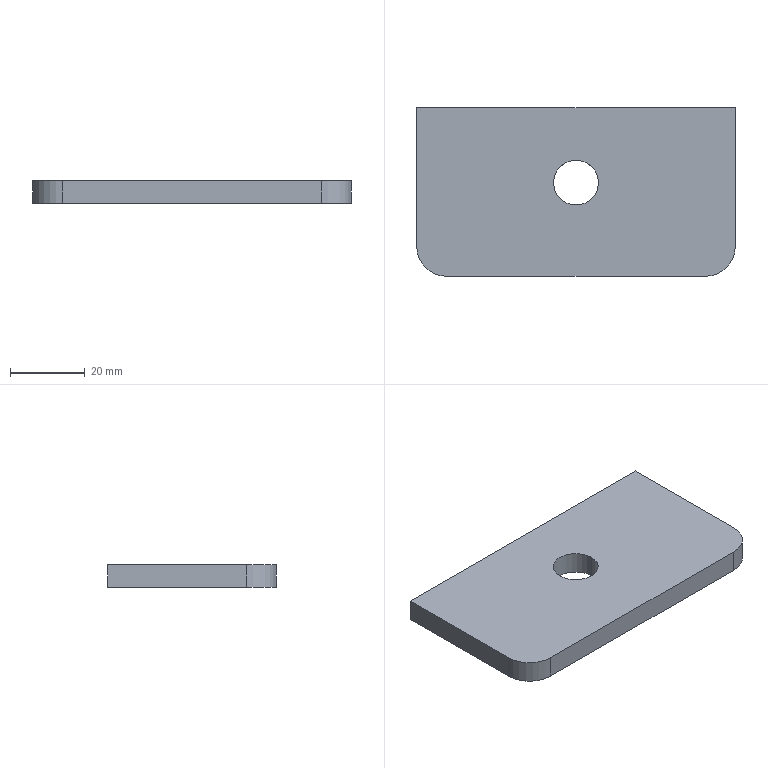Part | SolidWorks | features Extrusion 1 | 1 solid | 10 faces | box 85 x 45 x 6 mm | volume 22107 mm3 | plane 6 | cylinder 4 | commonest cylinder face diameters 12 x2 16 x2
STEP:
#1=CARTESIAN_POINT('',(-6.,2.5,6.));
#2=VERTEX_POINT('',#1);
#3=CARTESIAN_POINT('',(6.,2.5,6.));
#4=VERTEX_POINT('',#3);
#5=CARTESIAN_POINT('',(0.,2.5,6.));
#6=DIRECTION('',(0.,0.,1.));
#7=DIRECTION('',(1.,0.,0.));
#8=AXIS2_PLACEMENT_3D('',#5,#6,#7);
#9=CIRCLE('',#8,6.);
#10=EDGE_CURVE('',#2,#4,#9,.T.);
#11=ORIENTED_EDGE('',*,*,#10,.T.);
#12=CARTESIAN_POINT('',(6.,2.5,0.));
#13=VERTEX_POINT('',#12);
#14=CARTESIAN_POINT('',(6.,2.5,6.));
#15=DIRECTION('',(0.,0.,-1.));
#16=VECTOR('',#15,1000.);
#17=LINE('',#14,#16);
#18=EDGE_CURVE('',#4,#13,#17,.T.);
#19=ORIENTED_EDGE('',*,*,#18,.T.);
#20=CARTESIAN_POINT('',(-6.,2.5,0.));
#21=VERTEX_POINT('',#20);
#22=CARTESIAN_POINT('',(0.,2.5,0.));
#23=DIRECTION('',(0.,0.,1.));
#24=DIRECTION('',(1.,0.,0.));
#25=AXIS2_PLACEMENT_3D('',#22,#23,#24);
#26=CIRCLE('',#25,6.);
#27=EDGE_CURVE('',#21,#13,#26,.T.);
#28=ORIENTED_EDGE('',*,*,#27,.F.);
#29=CARTESIAN_POINT('',(-6.,2.5,6.));
#30=DIRECTION('',(0.,0.,-1.));
#31=VECTOR('',#30,1000.);
#32=LINE('',#29,#31);
#33=EDGE_CURVE('',#2,#21,#32,.T.);
#34=ORIENTED_EDGE('',*,*,#33,.F.);
#35=EDGE_LOOP('',(#11,#19,#28,#34));
#36=FACE_OUTER_BOUND('',#35,.T.);
#37=CARTESIAN_POINT('',(0.,2.5,6.));
#38=DIRECTION('',(0.,0.,-1.));
#39=DIRECTION('',(-1.,0.,0.));
#40=AXIS2_PLACEMENT_3D('',#37,#38,#39);
#41=CYLINDRICAL_SURFACE('',#40,6.);
#42=ADVANCED_FACE('',(#36),#41,.F.);
#43=CARTESIAN_POINT('',(-42.5,22.5,6.));
#44=VERTEX_POINT('',#43);
#45=CARTESIAN_POINT('',(-42.5,-14.5,6.));
#46=VERTEX_POINT('',#45);
#47=CARTESIAN_POINT('',(-42.5,22.5,6.));
#48=DIRECTION('',(0.,-1.,0.));
#49=VECTOR('',#48,1000.);
#50=LINE('',#47,#49);
#51=EDGE_CURVE('',#44,#46,#50,.T.);
#52=ORIENTED_EDGE('',*,*,#51,.T.);
#53=CARTESIAN_POINT('',(-34.5,-22.5,6.));
#54=VERTEX_POINT('',#53);
#55=CARTESIAN_POINT('',(-34.5,-14.5,6.));
#56=DIRECTION('',(0.,0.,1.));
#57=DIRECTION('',(1.,0.,0.));
#58=AXIS2_PLACEMENT_3D('',#55,#56,#57);
#59=CIRCLE('',#58,8.);
#60=EDGE_CURVE('',#46,#54,#59,.T.);
#61=ORIENTED_EDGE('',*,*,#60,.T.);
#62=CARTESIAN_POINT('',(34.5,-22.5,6.));
#63=VERTEX_POINT('',#62);
#64=CARTESIAN_POINT('',(-34.5,-22.5,6.));
#65=DIRECTION('',(1.,0.,0.));
#66=VECTOR('',#65,1000.);
#67=LINE('',#64,#66);
#68=EDGE_CURVE('',#54,#63,#67,.T.);
#69=ORIENTED_EDGE('',*,*,#68,.T.);
#70=CARTESIAN_POINT('',(42.5,-14.5,6.));
#71=VERTEX_POINT('',#70);
#72=CARTESIAN_POINT('',(34.5,-14.5,6.));
#73=DIRECTION('',(0.,0.,1.));
#74=DIRECTION('',(1.,0.,0.));
#75=AXIS2_PLACEMENT_3D('',#72,#73,#74);
#76=CIRCLE('',#75,8.);
#77=EDGE_CURVE('',#63,#71,#76,.T.);
#78=ORIENTED_EDGE('',*,*,#77,.T.);
#79=CARTESIAN_POINT('',(42.5,22.5,6.));
#80=VERTEX_POINT('',#79);
#81=CARTESIAN_POINT('',(42.5,22.5,6.));
#82=DIRECTION('',(0.,1.,0.));
#83=VECTOR('',#82,1000.);
#84=LINE('',#81,#83);
#85=EDGE_CURVE('',#71,#80,#84,.T.);
#86=ORIENTED_EDGE('',*,*,#85,.T.);
#87=CARTESIAN_POINT('',(-42.5,22.5,6.));
#88=DIRECTION('',(-1.,0.,0.));
#89=VECTOR('',#88,1000.);
#90=LINE('',#87,#89);
#91=EDGE_CURVE('',#80,#44,#90,.T.);
#92=ORIENTED_EDGE('',*,*,#91,.T.);
#93=EDGE_LOOP('',(#52,#61,#69,#78,#86,#92));
#94=FACE_OUTER_BOUND('',#93,.T.);
#95=ORIENTED_EDGE('',*,*,#10,.F.);
#96=CARTESIAN_POINT('',(0.,2.5,6.));
#97=DIRECTION('',(0.,0.,1.));
#98=DIRECTION('',(1.,0.,0.));
#99=AXIS2_PLACEMENT_3D('',#96,#97,#98);
#100=CIRCLE('',#99,6.);
#101=EDGE_CURVE('',#4,#2,#100,.T.);
#102=ORIENTED_EDGE('',*,*,#101,.F.);
#103=EDGE_LOOP('',(#95,#102));
#104=FACE_BOUND('',#103,.T.);
#105=CARTESIAN_POINT('',(-34.5,-14.5,6.));
#106=DIRECTION('',(0.,0.,1.));
#107=DIRECTION('',(1.,0.,0.));
#108=AXIS2_PLACEMENT_3D('',#105,#106,#107);
#109=PLANE('',#108);
#110=ADVANCED_FACE('',(#94,#104),#109,.T.);
#111=CARTESIAN_POINT('',(-42.5,22.5,0.));
#112=VERTEX_POINT('',#111);
#113=CARTESIAN_POINT('',(-42.5,-14.5,0.));
#114=VERTEX_POINT('',#113);
#115=CARTESIAN_POINT('',(-42.5,22.5,0.));
#116=DIRECTION('',(0.,-1.,0.));
#117=VECTOR('',#116,1000.);
#118=LINE('',#115,#117);
#119=EDGE_CURVE('',#112,#114,#118,.T.);
#120=ORIENTED_EDGE('',*,*,#119,.F.);
#121=CARTESIAN_POINT('',(42.5,22.5,0.));
#122=VERTEX_POINT('',#121);
#123=CARTESIAN_POINT('',(-42.5,22.5,0.));
#124=DIRECTION('',(-1.,0.,0.));
#125=VECTOR('',#124,1000.);
#126=LINE('',#123,#125);
#127=EDGE_CURVE('',#122,#112,#126,.T.);
#128=ORIENTED_EDGE('',*,*,#127,.F.);
#129=CARTESIAN_POINT('',(42.5,-14.5,0.));
#130=VERTEX_POINT('',#129);
#131=CARTESIAN_POINT('',(42.5,22.5,0.));
#132=DIRECTION('',(0.,1.,0.));
#133=VECTOR('',#132,1000.);
#134=LINE('',#131,#133);
#135=EDGE_CURVE('',#130,#122,#134,.T.);
#136=ORIENTED_EDGE('',*,*,#135,.F.);
#137=CARTESIAN_POINT('',(34.5,-22.5,0.));
#138=VERTEX_POINT('',#137);
#139=CARTESIAN_POINT('',(34.5,-14.5,0.));
#140=DIRECTION('',(0.,0.,1.));
#141=DIRECTION('',(1.,0.,0.));
#142=AXIS2_PLACEMENT_3D('',#139,#140,#141);
#143=CIRCLE('',#142,8.);
#144=EDGE_CURVE('',#138,#130,#143,.T.);
#145=ORIENTED_EDGE('',*,*,#144,.F.);
#146=CARTESIAN_POINT('',(-34.5,-22.5,0.));
#147=VERTEX_POINT('',#146);
#148=CARTESIAN_POINT('',(-34.5,-22.5,0.));
#149=DIRECTION('',(1.,0.,0.));
#150=VECTOR('',#149,1000.);
#151=LINE('',#148,#150);
#152=EDGE_CURVE('',#147,#138,#151,.T.);
#153=ORIENTED_EDGE('',*,*,#152,.F.);
#154=CARTESIAN_POINT('',(-34.5,-14.5,0.));
#155=DIRECTION('',(0.,0.,1.));
#156=DIRECTION('',(1.,0.,0.));
#157=AXIS2_PLACEMENT_3D('',#154,#155,#156);
#158=CIRCLE('',#157,8.);
#159=EDGE_CURVE('',#114,#147,#158,.T.);
#160=ORIENTED_EDGE('',*,*,#159,.F.);
#161=EDGE_LOOP('',(#120,#128,#136,#145,#153,#160));
#162=FACE_OUTER_BOUND('',#161,.T.);
#163=ORIENTED_EDGE('',*,*,#27,.T.);
#164=CARTESIAN_POINT('',(0.,2.5,0.));
#165=DIRECTION('',(0.,0.,1.));
#166=DIRECTION('',(1.,0.,0.));
#167=AXIS2_PLACEMENT_3D('',#164,#165,#166);
#168=CIRCLE('',#167,6.);
#169=EDGE_CURVE('',#13,#21,#168,.T.);
#170=ORIENTED_EDGE('',*,*,#169,.T.);
#171=EDGE_LOOP('',(#163,#170));
#172=FACE_BOUND('',#171,.T.);
#173=CARTESIAN_POINT('',(-34.5,-14.5,0.));
#174=DIRECTION('',(0.,0.,1.));
#175=DIRECTION('',(1.,0.,0.));
#176=AXIS2_PLACEMENT_3D('',#173,#174,#175);
#177=PLANE('',#176);
#178=ADVANCED_FACE('',(#162,#172),#177,.F.);
#179=ORIENTED_EDGE('',*,*,#119,.T.);
#180=CARTESIAN_POINT('',(-42.5,-14.5,6.));
#181=DIRECTION('',(0.,0.,-1.));
#182=VECTOR('',#181,1000.);
#183=LINE('',#180,#182);
#184=EDGE_CURVE('',#46,#114,#183,.T.);
#185=ORIENTED_EDGE('',*,*,#184,.F.);
#186=ORIENTED_EDGE('',*,*,#51,.F.);
#187=CARTESIAN_POINT('',(-42.5,22.5,6.));
#188=DIRECTION('',(0.,0.,-1.));
#189=VECTOR('',#188,1000.);
#190=LINE('',#187,#189);
#191=EDGE_CURVE('',#44,#112,#190,.T.);
#192=ORIENTED_EDGE('',*,*,#191,.T.);
#193=EDGE_LOOP('',(#179,#185,#186,#192));
#194=FACE_OUTER_BOUND('',#193,.T.);
#195=CARTESIAN_POINT('',(-42.5,22.5,6.));
#196=DIRECTION('',(1.,0.,0.));
#197=DIRECTION('',(0.,1.,0.));
#198=AXIS2_PLACEMENT_3D('',#195,#196,#197);
#199=PLANE('',#198);
#200=ADVANCED_FACE('',(#194),#199,.F.);
#201=ORIENTED_EDGE('',*,*,#159,.T.);
#202=CARTESIAN_POINT('',(-34.5,-22.5,6.));
#203=DIRECTION('',(0.,0.,-1.));
#204=VECTOR('',#203,1000.);
#205=LINE('',#202,#204);
#206=EDGE_CURVE('',#54,#147,#205,.T.);
#207=ORIENTED_EDGE('',*,*,#206,.F.);
#208=ORIENTED_EDGE('',*,*,#60,.F.);
#209=ORIENTED_EDGE('',*,*,#184,.T.);
#210=EDGE_LOOP('',(#201,#207,#208,#209));
#211=FACE_OUTER_BOUND('',#210,.T.);
#212=CARTESIAN_POINT('',(-34.5,-14.5,6.));
#213=DIRECTION('',(0.,0.,-1.));
#214=DIRECTION('',(-1.,0.,0.));
#215=AXIS2_PLACEMENT_3D('',#212,#213,#214);
#216=CYLINDRICAL_SURFACE('',#215,8.);
#217=ADVANCED_FACE('',(#211),#216,.T.);
#218=ORIENTED_EDGE('',*,*,#152,.T.);
#219=CARTESIAN_POINT('',(34.5,-22.5,6.));
#220=DIRECTION('',(0.,0.,-1.));
#221=VECTOR('',#220,1000.);
#222=LINE('',#219,#221);
#223=EDGE_CURVE('',#63,#138,#222,.T.);
#224=ORIENTED_EDGE('',*,*,#223,.F.);
#225=ORIENTED_EDGE('',*,*,#68,.F.);
#226=ORIENTED_EDGE('',*,*,#206,.T.);
#227=EDGE_LOOP('',(#218,#224,#225,#226));
#228=FACE_OUTER_BOUND('',#227,.T.);
#229=CARTESIAN_POINT('',(-34.5,-22.5,6.));
#230=DIRECTION('',(0.,1.,0.));
#231=DIRECTION('',(0.,0.,1.));
#232=AXIS2_PLACEMENT_3D('',#229,#230,#231);
#233=PLANE('',#232);
#234=ADVANCED_FACE('',(#228),#233,.F.);
#235=ORIENTED_EDGE('',*,*,#144,.T.);
#236=CARTESIAN_POINT('',(42.5,-14.5,6.));
#237=DIRECTION('',(0.,0.,-1.));
#238=VECTOR('',#237,1000.);
#239=LINE('',#236,#238);
#240=EDGE_CURVE('',#71,#130,#239,.T.);
#241=ORIENTED_EDGE('',*,*,#240,.F.);
#242=ORIENTED_EDGE('',*,*,#77,.F.);
#243=ORIENTED_EDGE('',*,*,#223,.T.);
#244=EDGE_LOOP('',(#235,#241,#242,#243));
#245=FACE_OUTER_BOUND('',#244,.T.);
#246=CARTESIAN_POINT('',(34.5,-14.5,6.));
#247=DIRECTION('',(0.,0.,-1.));
#248=DIRECTION('',(-1.,0.,0.));
#249=AXIS2_PLACEMENT_3D('',#246,#247,#248);
#250=CYLINDRICAL_SURFACE('',#249,8.);
#251=ADVANCED_FACE('',(#245),#250,.T.);
#252=ORIENTED_EDGE('',*,*,#135,.T.);
#253=CARTESIAN_POINT('',(42.5,22.5,6.));
#254=DIRECTION('',(0.,0.,-1.));
#255=VECTOR('',#254,1000.);
#256=LINE('',#253,#255);
#257=EDGE_CURVE('',#80,#122,#256,.T.);
#258=ORIENTED_EDGE('',*,*,#257,.F.);
#259=ORIENTED_EDGE('',*,*,#85,.F.);
#260=ORIENTED_EDGE('',*,*,#240,.T.);
#261=EDGE_LOOP('',(#252,#258,#259,#260));
#262=FACE_OUTER_BOUND('',#261,.T.);
#263=CARTESIAN_POINT('',(42.5,22.5,6.));
#264=DIRECTION('',(-1.,0.,0.));
#265=DIRECTION('',(0.,0.,1.));
#266=AXIS2_PLACEMENT_3D('',#263,#264,#265);
#267=PLANE('',#266);
#268=ADVANCED_FACE('',(#262),#267,.F.);
#269=ORIENTED_EDGE('',*,*,#127,.T.);
#270=ORIENTED_EDGE('',*,*,#191,.F.);
#271=ORIENTED_EDGE('',*,*,#91,.F.);
#272=ORIENTED_EDGE('',*,*,#257,.T.);
#273=EDGE_LOOP('',(#269,#270,#271,#272));
#274=FACE_OUTER_BOUND('',#273,.T.);
#275=CARTESIAN_POINT('',(-42.5,22.5,6.));
#276=DIRECTION('',(0.,-1.,0.));
#277=DIRECTION('',(0.,0.,-1.));
#278=AXIS2_PLACEMENT_3D('',#275,#276,#277);
#279=PLANE('',#278);
#280=ADVANCED_FACE('',(#274),#279,.F.);
#281=ORIENTED_EDGE('',*,*,#18,.F.);
#282=ORIENTED_EDGE('',*,*,#101,.T.);
#283=ORIENTED_EDGE('',*,*,#33,.T.);
#284=ORIENTED_EDGE('',*,*,#169,.F.);
#285=EDGE_LOOP('',(#281,#282,#283,#284));
#286=FACE_OUTER_BOUND('',#285,.T.);
#287=CARTESIAN_POINT('',(0.,2.5,6.));
#288=DIRECTION('',(0.,0.,-1.));
#289=DIRECTION('',(-1.,0.,0.));
#290=AXIS2_PLACEMENT_3D('',#287,#288,#289);
#291=CYLINDRICAL_SURFACE('',#290,6.);
#292=ADVANCED_FACE('',(#286),#291,.F.);
#293=CLOSED_SHELL('',(#42,#110,#178,#200,#217,#234,#251,#268,#280,#292));
#294=MANIFOLD_SOLID_BREP('',#293);
#295=CARTESIAN_POINT('',(0.,0.,0.));
#296=DIRECTION('',(0.,0.,1.));
#297=DIRECTION('',(1.,0.,0.));
#298=AXIS2_PLACEMENT_3D('',#295,#296,#297);
#299=(LENGTH_UNIT()NAMED_UNIT(*)SI_UNIT(.MILLI.,.METRE.));
#300=UNCERTAINTY_MEASURE_WITH_UNIT(LENGTH_MEASURE(0.00001),#299,'','');
#301=(NAMED_UNIT(*)PLANE_ANGLE_UNIT()SI_UNIT($,.RADIAN.));
#302=(NAMED_UNIT(*)SI_UNIT($,.STERADIAN.)SOLID_ANGLE_UNIT());
#303=(GEOMETRIC_REPRESENTATION_CONTEXT(3)GLOBAL_UNCERTAINTY_ASSIGNED_CONTEXT((#300))GLOBAL_UNIT_ASSIGNED_CONTEXT((#299,#301,#302))REPRESENTATION_CONTEXT('',''));
#304=ADVANCED_BREP_SHAPE_REPRESENTATION('',(#294,#298),#303);